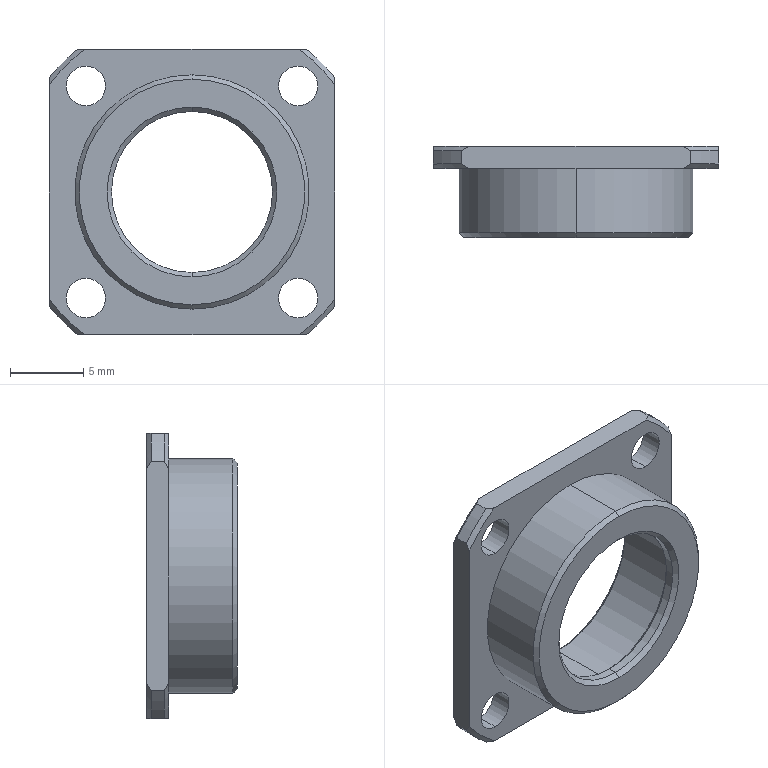Part | SolidWorks | features ICE 2, Revolution 1 | 1 solid | 42 faces | box 19.5 x 6.2 x 19.5 mm | volume 684.644 mm3 | cylinder 18 | cone 16 | plane 8 | commonest cylinder face diameters 2.7 x8 25 x4 11 x2 13 x2 16 x2
STEP:
#1=CARTESIAN_POINT('',(-7.25,4.7,8.6));
#2=VERTEX_POINT('',#1);
#3=CARTESIAN_POINT('',(-7.25,4.7,5.9));
#4=VERTEX_POINT('',#3);
#5=CARTESIAN_POINT('',(-7.25,4.7,7.25));
#6=DIRECTION('',(0.,-1.,0.));
#7=DIRECTION('',(0.,0.,-1.));
#8=AXIS2_PLACEMENT_3D('',#5,#6,#7);
#9=CIRCLE('',#8,1.35);
#10=EDGE_CURVE('',#2,#4,#9,.T.);
#11=ORIENTED_EDGE('',*,*,#10,.T.);
#12=CARTESIAN_POINT('',(-7.25,6.2,5.9));
#13=VERTEX_POINT('',#12);
#14=CARTESIAN_POINT('',(-7.25,-3.8,5.9));
#15=DIRECTION('',(0.,1.,0.));
#16=VECTOR('',#15,1000.);
#17=LINE('',#14,#16);
#18=EDGE_CURVE('',#4,#13,#17,.T.);
#19=ORIENTED_EDGE('',*,*,#18,.T.);
#20=CARTESIAN_POINT('',(-7.25,6.2,8.6));
#21=VERTEX_POINT('',#20);
#22=CARTESIAN_POINT('',(-7.25,6.2,7.25));
#23=DIRECTION('',(0.,1.,0.));
#24=DIRECTION('',(0.,0.,-1.));
#25=AXIS2_PLACEMENT_3D('',#22,#23,#24);
#26=CIRCLE('',#25,1.35);
#27=EDGE_CURVE('',#13,#21,#26,.T.);
#28=ORIENTED_EDGE('',*,*,#27,.T.);
#29=CARTESIAN_POINT('',(-7.25,-3.8,8.6));
#30=DIRECTION('',(0.,1.,0.));
#31=VECTOR('',#30,1000.);
#32=LINE('',#29,#31);
#33=EDGE_CURVE('',#2,#21,#32,.T.);
#34=ORIENTED_EDGE('',*,*,#33,.F.);
#35=EDGE_LOOP('',(#11,#19,#28,#34));
#36=FACE_OUTER_BOUND('',#35,.T.);
#37=CARTESIAN_POINT('',(-7.25,-3.8,7.25));
#38=DIRECTION('',(0.,1.,0.));
#39=DIRECTION('',(0.,0.,1.));
#40=AXIS2_PLACEMENT_3D('',#37,#38,#39);
#41=CYLINDRICAL_SURFACE('',#40,1.35);
#42=ADVANCED_FACE('',(#36),#41,.F.);
#43=CARTESIAN_POINT('',(7.25,4.7,8.6));
#44=VERTEX_POINT('',#43);
#45=CARTESIAN_POINT('',(7.25,4.7,5.9));
#46=VERTEX_POINT('',#45);
#47=CARTESIAN_POINT('',(7.25,4.7,7.25));
#48=DIRECTION('',(0.,-1.,0.));
#49=DIRECTION('',(0.,0.,-1.));
#50=AXIS2_PLACEMENT_3D('',#47,#48,#49);
#51=CIRCLE('',#50,1.35);
#52=EDGE_CURVE('',#44,#46,#51,.T.);
#53=ORIENTED_EDGE('',*,*,#52,.T.);
#54=CARTESIAN_POINT('',(7.25,6.2,5.9));
#55=VERTEX_POINT('',#54);
#56=CARTESIAN_POINT('',(7.25,-3.8,5.9));
#57=DIRECTION('',(0.,1.,0.));
#58=VECTOR('',#57,1000.);
#59=LINE('',#56,#58);
#60=EDGE_CURVE('',#46,#55,#59,.T.);
#61=ORIENTED_EDGE('',*,*,#60,.T.);
#62=CARTESIAN_POINT('',(7.25,6.2,8.6));
#63=VERTEX_POINT('',#62);
#64=CARTESIAN_POINT('',(7.25,6.2,7.25));
#65=DIRECTION('',(0.,1.,0.));
#66=DIRECTION('',(0.,0.,1.));
#67=AXIS2_PLACEMENT_3D('',#64,#65,#66);
#68=CIRCLE('',#67,1.35);
#69=EDGE_CURVE('',#55,#63,#68,.T.);
#70=ORIENTED_EDGE('',*,*,#69,.T.);
#71=CARTESIAN_POINT('',(7.25,-3.8,8.6));
#72=DIRECTION('',(0.,1.,0.));
#73=VECTOR('',#72,1000.);
#74=LINE('',#71,#73);
#75=EDGE_CURVE('',#44,#63,#74,.T.);
#76=ORIENTED_EDGE('',*,*,#75,.F.);
#77=EDGE_LOOP('',(#53,#61,#70,#76));
#78=FACE_OUTER_BOUND('',#77,.T.);
#79=CARTESIAN_POINT('',(7.25,-3.8,7.25));
#80=DIRECTION('',(0.,1.,0.));
#81=DIRECTION('',(0.,0.,1.));
#82=AXIS2_PLACEMENT_3D('',#79,#80,#81);
#83=CYLINDRICAL_SURFACE('',#82,1.35);
#84=ADVANCED_FACE('',(#78),#83,.F.);
#85=CARTESIAN_POINT('',(7.25,4.7,-5.9));
#86=VERTEX_POINT('',#85);
#87=CARTESIAN_POINT('',(7.25,4.7,-8.6));
#88=VERTEX_POINT('',#87);
#89=CARTESIAN_POINT('',(7.25,4.7,-7.25));
#90=DIRECTION('',(0.,-1.,0.));
#91=DIRECTION('',(0.,0.,-1.));
#92=AXIS2_PLACEMENT_3D('',#89,#90,#91);
#93=CIRCLE('',#92,1.35);
#94=EDGE_CURVE('',#86,#88,#93,.T.);
#95=ORIENTED_EDGE('',*,*,#94,.T.);
#96=CARTESIAN_POINT('',(7.25,6.2,-8.6));
#97=VERTEX_POINT('',#96);
#98=CARTESIAN_POINT('',(7.25,-3.8,-8.6));
#99=DIRECTION('',(0.,1.,0.));
#100=VECTOR('',#99,1000.);
#101=LINE('',#98,#100);
#102=EDGE_CURVE('',#88,#97,#101,.T.);
#103=ORIENTED_EDGE('',*,*,#102,.T.);
#104=CARTESIAN_POINT('',(7.25,6.2,-5.9));
#105=VERTEX_POINT('',#104);
#106=CARTESIAN_POINT('',(7.25,6.2,-7.25));
#107=DIRECTION('',(0.,1.,0.));
#108=DIRECTION('',(0.,0.,-1.));
#109=AXIS2_PLACEMENT_3D('',#106,#107,#108);
#110=CIRCLE('',#109,1.35);
#111=EDGE_CURVE('',#97,#105,#110,.T.);
#112=ORIENTED_EDGE('',*,*,#111,.T.);
#113=CARTESIAN_POINT('',(7.25,-3.8,-5.9));
#114=DIRECTION('',(0.,1.,0.));
#115=VECTOR('',#114,1000.);
#116=LINE('',#113,#115);
#117=EDGE_CURVE('',#86,#105,#116,.T.);
#118=ORIENTED_EDGE('',*,*,#117,.F.);
#119=EDGE_LOOP('',(#95,#103,#112,#118));
#120=FACE_OUTER_BOUND('',#119,.T.);
#121=CARTESIAN_POINT('',(7.25,-3.8,-7.25));
#122=DIRECTION('',(0.,1.,0.));
#123=DIRECTION('',(0.,0.,1.));
#124=AXIS2_PLACEMENT_3D('',#121,#122,#123);
#125=CYLINDRICAL_SURFACE('',#124,1.35);
#126=ADVANCED_FACE('',(#120),#125,.F.);
#127=CARTESIAN_POINT('',(-7.25,4.7,-5.9));
#128=VERTEX_POINT('',#127);
#129=CARTESIAN_POINT('',(-7.25,4.7,-8.6));
#130=VERTEX_POINT('',#129);
#131=CARTESIAN_POINT('',(-7.25,4.7,-7.25));
#132=DIRECTION('',(0.,-1.,0.));
#133=DIRECTION('',(0.,0.,-1.));
#134=AXIS2_PLACEMENT_3D('',#131,#132,#133);
#135=CIRCLE('',#134,1.35);
#136=EDGE_CURVE('',#128,#130,#135,.T.);
#137=ORIENTED_EDGE('',*,*,#136,.T.);
#138=CARTESIAN_POINT('',(-7.25,6.2,-8.6));
#139=VERTEX_POINT('',#138);
#140=CARTESIAN_POINT('',(-7.25,-3.8,-8.6));
#141=DIRECTION('',(0.,1.,0.));
#142=VECTOR('',#141,1000.);
#143=LINE('',#140,#142);
#144=EDGE_CURVE('',#130,#139,#143,.T.);
#145=ORIENTED_EDGE('',*,*,#144,.T.);
#146=CARTESIAN_POINT('',(-7.25,6.2,-5.9));
#147=VERTEX_POINT('',#146);
#148=CARTESIAN_POINT('',(-7.25,6.2,-7.25));
#149=DIRECTION('',(0.,1.,0.));
#150=DIRECTION('',(0.,0.,1.));
#151=AXIS2_PLACEMENT_3D('',#148,#149,#150);
#152=CIRCLE('',#151,1.35);
#153=EDGE_CURVE('',#139,#147,#152,.T.);
#154=ORIENTED_EDGE('',*,*,#153,.T.);
#155=CARTESIAN_POINT('',(-7.25,-3.8,-5.9));
#156=DIRECTION('',(0.,1.,0.));
#157=VECTOR('',#156,1000.);
#158=LINE('',#155,#157);
#159=EDGE_CURVE('',#128,#147,#158,.T.);
#160=ORIENTED_EDGE('',*,*,#159,.F.);
#161=EDGE_LOOP('',(#137,#145,#154,#160));
#162=FACE_OUTER_BOUND('',#161,.T.);
#163=CARTESIAN_POINT('',(-7.25,-3.8,-7.25));
#164=DIRECTION('',(0.,1.,0.));
#165=DIRECTION('',(0.,0.,1.));
#166=AXIS2_PLACEMENT_3D('',#163,#164,#165);
#167=CYLINDRICAL_SURFACE('',#166,1.35);
#168=ADVANCED_FACE('',(#162),#167,.F.);
#169=CARTESIAN_POINT('',(0.,4.7,-8.));
#170=VERTEX_POINT('',#169);
#171=CARTESIAN_POINT('',(0.,4.7,8.));
#172=VERTEX_POINT('',#171);
#173=CARTESIAN_POINT('',(0.,4.7,0.));
#174=DIRECTION('',(0.,-1.,0.));
#175=DIRECTION('',(0.,0.,-1.));
#176=AXIS2_PLACEMENT_3D('',#173,#174,#175);
#177=CIRCLE('',#176,8.);
#178=EDGE_CURVE('',#170,#172,#177,.T.);
#179=ORIENTED_EDGE('',*,*,#178,.T.);
#180=CARTESIAN_POINT('',(0.,0.3,8.));
#181=VERTEX_POINT('',#180);
#182=CARTESIAN_POINT('',(0.,0.,8.));
#183=DIRECTION('',(0.,-1.,0.));
#184=VECTOR('',#183,1000.);
#185=LINE('',#182,#184);
#186=EDGE_CURVE('',#172,#181,#185,.T.);
#187=ORIENTED_EDGE('',*,*,#186,.T.);
#188=CARTESIAN_POINT('',(0.,0.3,-8.));
#189=VERTEX_POINT('',#188);
#190=CARTESIAN_POINT('',(0.,0.3,0.));
#191=DIRECTION('',(0.,-1.,0.));
#192=DIRECTION('',(0.,0.,-1.));
#193=AXIS2_PLACEMENT_3D('',#190,#191,#192);
#194=CIRCLE('',#193,8.);
#195=EDGE_CURVE('',#189,#181,#194,.T.);
#196=ORIENTED_EDGE('',*,*,#195,.F.);
#197=CARTESIAN_POINT('',(0.,0.,-8.));
#198=DIRECTION('',(0.,-1.,0.));
#199=VECTOR('',#198,1000.);
#200=LINE('',#197,#199);
#201=EDGE_CURVE('',#170,#189,#200,.T.);
#202=ORIENTED_EDGE('',*,*,#201,.F.);
#203=EDGE_LOOP('',(#179,#187,#196,#202));
#204=FACE_OUTER_BOUND('',#203,.T.);
#205=CARTESIAN_POINT('',(0.,0.,0.));
#206=DIRECTION('',(0.,-1.,0.));
#207=DIRECTION('',(0.,0.,-1.));
#208=AXIS2_PLACEMENT_3D('',#205,#206,#207);
#209=CYLINDRICAL_SURFACE('',#208,8.);
#210=ADVANCED_FACE('',(#204),#209,.T.);
#211=CARTESIAN_POINT('',(0.,0.,-7.7));
#212=VERTEX_POINT('',#211);
#213=CARTESIAN_POINT('',(0.,0.,7.7));
#214=VERTEX_POINT('',#213);
#215=CARTESIAN_POINT('',(0.,0.,0.));
#216=DIRECTION('',(0.,-1.,0.));
#217=DIRECTION('',(0.,0.,-1.));
#218=AXIS2_PLACEMENT_3D('',#215,#216,#217);
#219=CIRCLE('',#218,7.7);
#220=EDGE_CURVE('',#212,#214,#219,.T.);
#221=ORIENTED_EDGE('',*,*,#220,.F.);
#222=CARTESIAN_POINT('',(0.,0.,-7.7));
#223=DIRECTION('',(0.,0.7071,-0.7071));
#224=VECTOR('',#223,1000.);
#225=LINE('',#222,#224);
#226=EDGE_CURVE('',#212,#189,#225,.T.);
#227=ORIENTED_EDGE('',*,*,#226,.T.);
#228=ORIENTED_EDGE('',*,*,#195,.T.);
#229=CARTESIAN_POINT('',(0.,0.,7.7));
#230=DIRECTION('',(0.,0.7071,0.7071));
#231=VECTOR('',#230,1000.);
#232=LINE('',#229,#231);
#233=EDGE_CURVE('',#214,#181,#232,.T.);
#234=ORIENTED_EDGE('',*,*,#233,.F.);
#235=EDGE_LOOP('',(#221,#227,#228,#234));
#236=FACE_OUTER_BOUND('',#235,.T.);
#237=CARTESIAN_POINT('',(0.,0.,0.));
#238=DIRECTION('',(0.,1.,0.));
#239=DIRECTION('',(0.,0.,1.));
#240=AXIS2_PLACEMENT_3D('',#237,#238,#239);
#241=CONICAL_SURFACE('',#240,7.7,0.7854);
#242=ADVANCED_FACE('',(#236),#241,.T.);
#243=CARTESIAN_POINT('',(0.,0.3,5.5));
#244=VERTEX_POINT('',#243);
#245=CARTESIAN_POINT('',(0.,0.3,-5.5));
#246=VERTEX_POINT('',#245);
#247=CARTESIAN_POINT('',(0.,0.3,0.));
#248=DIRECTION('',(0.,-1.,0.));
#249=DIRECTION('',(0.,0.,-1.));
#250=AXIS2_PLACEMENT_3D('',#247,#248,#249);
#251=CIRCLE('',#250,5.5);
#252=EDGE_CURVE('',#244,#246,#251,.T.);
#253=ORIENTED_EDGE('',*,*,#252,.F.);
#254=CARTESIAN_POINT('',(0.,0.,5.8));
#255=VERTEX_POINT('',#254);
#256=CARTESIAN_POINT('',(0.,0.3,5.5));
#257=DIRECTION('',(0.,-0.7071,0.7071));
#258=VECTOR('',#257,1000.);
#259=LINE('',#256,#258);
#260=EDGE_CURVE('',#244,#255,#259,.T.);
#261=ORIENTED_EDGE('',*,*,#260,.T.);
#262=CARTESIAN_POINT('',(0.,0.,-5.8));
#263=VERTEX_POINT('',#262);
#264=CARTESIAN_POINT('',(0.,0.,0.));
#265=DIRECTION('',(0.,-1.,0.));
#266=DIRECTION('',(0.,0.,-1.));
#267=AXIS2_PLACEMENT_3D('',#264,#265,#266);
#268=CIRCLE('',#267,5.8);
#269=EDGE_CURVE('',#255,#263,#268,.T.);
#270=ORIENTED_EDGE('',*,*,#269,.T.);
#271=CARTESIAN_POINT('',(0.,0.3,-5.5));
#272=DIRECTION('',(0.,-0.7071,-0.7071));
#273=VECTOR('',#272,1000.);
#274=LINE('',#271,#273);
#275=EDGE_CURVE('',#246,#263,#274,.T.);
#276=ORIENTED_EDGE('',*,*,#275,.F.);
#277=EDGE_LOOP('',(#253,#261,#270,#276));
#278=FACE_OUTER_BOUND('',#277,.T.);
#279=CARTESIAN_POINT('',(0.,0.3,0.));
#280=DIRECTION('',(0.,-1.,0.));
#281=DIRECTION('',(0.,0.,-1.));
#282=AXIS2_PLACEMENT_3D('',#279,#280,#281);
#283=CONICAL_SURFACE('',#282,5.5,0.7854);
#284=ADVANCED_FACE('',(#278),#283,.F.);
#285=CARTESIAN_POINT('',(0.,0.9,5.5));
#286=VERTEX_POINT('',#285);
#287=CARTESIAN_POINT('',(0.,0.9,-5.5));
#288=VERTEX_POINT('',#287);
#289=CARTESIAN_POINT('',(0.,0.9,0.));
#290=DIRECTION('',(0.,-1.,0.));
#291=DIRECTION('',(0.,0.,-1.));
#292=AXIS2_PLACEMENT_3D('',#289,#290,#291);
#293=CIRCLE('',#292,5.5);
#294=EDGE_CURVE('',#286,#288,#293,.T.);
#295=ORIENTED_EDGE('',*,*,#294,.F.);
#296=CARTESIAN_POINT('',(0.,0.,5.5));
#297=DIRECTION('',(0.,-1.,0.));
#298=VECTOR('',#297,1000.);
#299=LINE('',#296,#298);
#300=EDGE_CURVE('',#286,#244,#299,.T.);
#301=ORIENTED_EDGE('',*,*,#300,.T.);
#302=ORIENTED_EDGE('',*,*,#252,.T.);
#303=CARTESIAN_POINT('',(0.,0.,-5.5));
#304=DIRECTION('',(0.,-1.,0.));
#305=VECTOR('',#304,1000.);
#306=LINE('',#303,#305);
#307=EDGE_CURVE('',#288,#246,#306,.T.);
#308=ORIENTED_EDGE('',*,*,#307,.F.);
#309=EDGE_LOOP('',(#295,#301,#302,#308));
#310=FACE_OUTER_BOUND('',#309,.T.);
#311=CARTESIAN_POINT('',(0.,0.,0.));
#312=DIRECTION('',(0.,-1.,0.));
#313=DIRECTION('',(0.,0.,-1.));
#314=AXIS2_PLACEMENT_3D('',#311,#312,#313);
#315=CYLINDRICAL_SURFACE('',#314,5.5);
#316=ADVANCED_FACE('',(#310),#315,.F.);
#317=ORIENTED_EDGE('',*,*,#294,.T.);
#318=CARTESIAN_POINT('',(0.,1.2,-5.8));
#319=VERTEX_POINT('',#318);
#320=CARTESIAN_POINT('',(0.,1.2,-5.8));
#321=DIRECTION('',(0.,0.7071,-0.7071));
#322=VECTOR('',#321,1000.);
#323=LINE('',#320,#322);
#324=EDGE_CURVE('',#288,#319,#323,.T.);
#325=ORIENTED_EDGE('',*,*,#324,.T.);
#326=CARTESIAN_POINT('',(0.,1.2,5.8));
#327=VERTEX_POINT('',#326);
#328=CARTESIAN_POINT('',(0.,1.2,0.));
#329=DIRECTION('',(0.,-1.,0.));
#330=DIRECTION('',(0.,0.,-1.));
#331=AXIS2_PLACEMENT_3D('',#328,#329,#330);
#332=CIRCLE('',#331,5.8);
#333=EDGE_CURVE('',#327,#319,#332,.T.);
#334=ORIENTED_EDGE('',*,*,#333,.F.);
#335=CARTESIAN_POINT('',(0.,1.2,5.8));
#336=DIRECTION('',(0.,0.7071,0.7071));
#337=VECTOR('',#336,1000.);
#338=LINE('',#335,#337);
#339=EDGE_CURVE('',#286,#327,#338,.T.);
#340=ORIENTED_EDGE('',*,*,#339,.F.);
#341=EDGE_LOOP('',(#317,#325,#334,#340));
#342=FACE_OUTER_BOUND('',#341,.T.);
#343=CARTESIAN_POINT('',(0.,1.2,0.));
#344=DIRECTION('',(0.,1.,0.));
#345=DIRECTION('',(0.,0.,1.));
#346=AXIS2_PLACEMENT_3D('',#343,#344,#345);
#347=CONICAL_SURFACE('',#346,5.8,0.7854);
#348=ADVANCED_FACE('',(#342),#347,.F.);
#349=CARTESIAN_POINT('',(0.,5.9,6.5));
#350=VERTEX_POINT('',#349);
#351=CARTESIAN_POINT('',(0.,5.9,-6.5));
#352=VERTEX_POINT('',#351);
#353=CARTESIAN_POINT('',(0.,5.9,0.));
#354=DIRECTION('',(0.,-1.,0.));
#355=DIRECTION('',(0.,0.,-1.));
#356=AXIS2_PLACEMENT_3D('',#353,#354,#355);
#357=CIRCLE('',#356,6.5);
#358=EDGE_CURVE('',#350,#352,#357,.T.);
#359=ORIENTED_EDGE('',*,*,#358,.F.);
#360=CARTESIAN_POINT('',(0.,1.2,6.5));
#361=VERTEX_POINT('',#360);
#362=CARTESIAN_POINT('',(0.,0.,6.5));
#363=DIRECTION('',(0.,-1.,0.));
#364=VECTOR('',#363,1000.);
#365=LINE('',#362,#364);
#366=EDGE_CURVE('',#350,#361,#365,.T.);
#367=ORIENTED_EDGE('',*,*,#366,.T.);
#368=CARTESIAN_POINT('',(0.,1.2,-6.5));
#369=VERTEX_POINT('',#368);
#370=CARTESIAN_POINT('',(0.,1.2,0.));
#371=DIRECTION('',(0.,-1.,0.));
#372=DIRECTION('',(0.,0.,-1.));
#373=AXIS2_PLACEMENT_3D('',#370,#371,#372);
#374=CIRCLE('',#373,6.5);
#375=EDGE_CURVE('',#361,#369,#374,.T.);
#376=ORIENTED_EDGE('',*,*,#375,.T.);
#377=CARTESIAN_POINT('',(0.,0.,-6.5));
#378=DIRECTION('',(0.,-1.,0.));
#379=VECTOR('',#378,1000.);
#380=LINE('',#377,#379);
#381=EDGE_CURVE('',#352,#369,#380,.T.);
#382=ORIENTED_EDGE('',*,*,#381,.F.);
#383=EDGE_LOOP('',(#359,#367,#376,#382));
#384=FACE_OUTER_BOUND('',#383,.T.);
#385=CARTESIAN_POINT('',(0.,0.,0.));
#386=DIRECTION('',(0.,-1.,0.));
#387=DIRECTION('',(0.,0.,-1.));
#388=AXIS2_PLACEMENT_3D('',#385,#386,#387);
#389=CYLINDRICAL_SURFACE('',#388,6.5);
#390=ADVANCED_FACE('',(#384),#389,.F.);
#391=ORIENTED_EDGE('',*,*,#358,.T.);
#392=CARTESIAN_POINT('',(0.,6.2,-6.8));
#393=VERTEX_POINT('',#392);
#394=CARTESIAN_POINT('',(0.,6.2,-6.8));
#395=DIRECTION('',(0.,0.7071,-0.7071));
#396=VECTOR('',#395,1000.);
#397=LINE('',#394,#396);
#398=EDGE_CURVE('',#352,#393,#397,.T.);
#399=ORIENTED_EDGE('',*,*,#398,.T.);
#400=CARTESIAN_POINT('',(0.,6.2,6.8));
#401=VERTEX_POINT('',#400);
#402=CARTESIAN_POINT('',(0.,6.2,0.));
#403=DIRECTION('',(0.,-1.,0.));
#404=DIRECTION('',(0.,0.,-1.));
#405=AXIS2_PLACEMENT_3D('',#402,#403,#404);
#406=CIRCLE('',#405,6.8);
#407=EDGE_CURVE('',#401,#393,#406,.T.);
#408=ORIENTED_EDGE('',*,*,#407,.F.);
#409=CARTESIAN_POINT('',(0.,6.2,6.8));
#410=DIRECTION('',(0.,0.7071,0.7071));
#411=VECTOR('',#410,1000.);
#412=LINE('',#409,#411);
#413=EDGE_CURVE('',#350,#401,#412,.T.);
#414=ORIENTED_EDGE('',*,*,#413,.F.);
#415=EDGE_LOOP('',(#391,#399,#408,#414));
#416=FACE_OUTER_BOUND('',#415,.T.);
#417=CARTESIAN_POINT('',(0.,6.2,0.));
#418=DIRECTION('',(0.,1.,0.));
#419=DIRECTION('',(0.,0.,1.));
#420=AXIS2_PLACEMENT_3D('',#417,#418,#419);
#421=CONICAL_SURFACE('',#420,6.8,0.7854);
#422=ADVANCED_FACE('',(#416),#421,.F.);
#423=ORIENTED_EDGE('',*,*,#10,.F.);
#424=CARTESIAN_POINT('',(-7.25,4.7,7.25));
#425=DIRECTION('',(0.,-1.,0.));
#426=DIRECTION('',(0.,0.,-1.));
#427=AXIS2_PLACEMENT_3D('',#424,#425,#426);
#428=CIRCLE('',#427,1.35);
#429=EDGE_CURVE('',#4,#2,#428,.T.);
#430=ORIENTED_EDGE('',*,*,#429,.F.);
#431=EDGE_LOOP('',(#423,#430));
#432=FACE_BOUND('',#431,.T.);
#433=ORIENTED_EDGE('',*,*,#52,.F.);
#434=CARTESIAN_POINT('',(7.25,4.7,7.25));
#435=DIRECTION('',(0.,-1.,0.));
#436=DIRECTION('',(0.,0.,-1.));
#437=AXIS2_PLACEMENT_3D('',#434,#435,#436);
#438=CIRCLE('',#437,1.35);
#439=EDGE_CURVE('',#46,#44,#438,.T.);
#440=ORIENTED_EDGE('',*,*,#439,.F.);
#441=EDGE_LOOP('',(#433,#440));
#442=FACE_BOUND('',#441,.T.);
#443=ORIENTED_EDGE('',*,*,#94,.F.);
#444=CARTESIAN_POINT('',(7.25,4.7,-7.25));
#445=DIRECTION('',(0.,-1.,0.));
#446=DIRECTION('',(0.,0.,-1.));
#447=AXIS2_PLACEMENT_3D('',#444,#445,#446);
#448=CIRCLE('',#447,1.35);
#449=EDGE_CURVE('',#88,#86,#448,.T.);
#450=ORIENTED_EDGE('',*,*,#449,.F.);
#451=EDGE_LOOP('',(#443,#450));
#452=FACE_BOUND('',#451,.T.);
#453=ORIENTED_EDGE('',*,*,#136,.F.);
#454=CARTESIAN_POINT('',(-7.25,4.7,-7.25));
#455=DIRECTION('',(0.,-1.,0.));
#456=DIRECTION('',(0.,0.,-1.));
#457=AXIS2_PLACEMENT_3D('',#454,#455,#456);
#458=CIRCLE('',#457,1.35);
#459=EDGE_CURVE('',#130,#128,#458,.T.);
#460=ORIENTED_EDGE('',*,*,#459,.F.);
#461=EDGE_LOOP('',(#453,#460));
#462=FACE_BOUND('',#461,.T.);
#463=ORIENTED_EDGE('',*,*,#178,.F.);
#464=CARTESIAN_POINT('',(0.,4.7,0.));
#465=DIRECTION('',(0.,-1.,0.));
#466=DIRECTION('',(0.,0.,-1.));
#467=AXIS2_PLACEMENT_3D('',#464,#465,#466);
#468=CIRCLE('',#467,8.);
#469=EDGE_CURVE('',#172,#170,#468,.T.);
#470=ORIENTED_EDGE('',*,*,#469,.F.);
#471=EDGE_LOOP('',(#463,#470));
#472=FACE_BOUND('',#471,.T.);
#473=CARTESIAN_POINT('',(7.333,4.7,-9.75));
#474=VERTEX_POINT('',#473);
#475=CARTESIAN_POINT('',(9.75,4.7,-7.333));
#476=VERTEX_POINT('',#475);
#477=CARTESIAN_POINT('',(0.,4.7,0.));
#478=DIRECTION('',(0.,-1.,0.));
#479=DIRECTION('',(0.,0.,-1.));
#480=AXIS2_PLACEMENT_3D('',#477,#478,#479);
#481=CIRCLE('',#480,12.2);
#482=EDGE_CURVE('',#474,#476,#481,.T.);
#483=ORIENTED_EDGE('',*,*,#482,.T.);
#484=CARTESIAN_POINT('',(9.75,4.7,7.333));
#485=VERTEX_POINT('',#484);
#486=CARTESIAN_POINT('',(9.75,4.7,0.));
#487=DIRECTION('',(0.,0.,1.));
#488=VECTOR('',#487,1000.);
#489=LINE('',#486,#488);
#490=EDGE_CURVE('',#476,#485,#489,.T.);
#491=ORIENTED_EDGE('',*,*,#490,.T.);
#492=CARTESIAN_POINT('',(7.333,4.7,9.75));
#493=VERTEX_POINT('',#492);
#494=CARTESIAN_POINT('',(0.,4.7,0.));
#495=DIRECTION('',(0.,-1.,0.));
#496=DIRECTION('',(0.,0.,-1.));
#497=AXIS2_PLACEMENT_3D('',#494,#495,#496);
#498=CIRCLE('',#497,12.2);
#499=EDGE_CURVE('',#485,#493,#498,.T.);
#500=ORIENTED_EDGE('',*,*,#499,.T.);
#501=CARTESIAN_POINT('',(-7.333,4.7,9.75));
#502=VERTEX_POINT('',#501);
#503=CARTESIAN_POINT('',(8.,4.7,9.75));
#504=DIRECTION('',(-1.,0.,0.));
#505=VECTOR('',#504,1000.);
#506=LINE('',#503,#505);
#507=EDGE_CURVE('',#493,#502,#506,.T.);
#508=ORIENTED_EDGE('',*,*,#507,.T.);
#509=CARTESIAN_POINT('',(-9.75,4.7,7.333));
#510=VERTEX_POINT('',#509);
#511=CARTESIAN_POINT('',(0.,4.7,0.));
#512=DIRECTION('',(0.,-1.,0.));
#513=DIRECTION('',(0.,0.,-1.));
#514=AXIS2_PLACEMENT_3D('',#511,#512,#513);
#515=CIRCLE('',#514,12.2);
#516=EDGE_CURVE('',#502,#510,#515,.T.);
#517=ORIENTED_EDGE('',*,*,#516,.T.);
#518=CARTESIAN_POINT('',(-9.75,4.7,-7.333));
#519=VERTEX_POINT('',#518);
#520=CARTESIAN_POINT('',(-9.75,4.7,0.));
#521=DIRECTION('',(0.,0.,-1.));
#522=VECTOR('',#521,1000.);
#523=LINE('',#520,#522);
#524=EDGE_CURVE('',#510,#519,#523,.T.);
#525=ORIENTED_EDGE('',*,*,#524,.T.);
#526=CARTESIAN_POINT('',(-7.333,4.7,-9.75));
#527=VERTEX_POINT('',#526);
#528=CARTESIAN_POINT('',(0.,4.7,0.));
#529=DIRECTION('',(0.,-1.,0.));
#530=DIRECTION('',(0.,0.,-1.));
#531=AXIS2_PLACEMENT_3D('',#528,#529,#530);
#532=CIRCLE('',#531,12.2);
#533=EDGE_CURVE('',#519,#527,#532,.T.);
#534=ORIENTED_EDGE('',*,*,#533,.T.);
#535=CARTESIAN_POINT('',(8.,4.7,-9.75));
#536=DIRECTION('',(1.,0.,0.));
#537=VECTOR('',#536,1000.);
#538=LINE('',#535,#537);
#539=EDGE_CURVE('',#527,#474,#538,.T.);
#540=ORIENTED_EDGE('',*,*,#539,.T.);
#541=EDGE_LOOP('',(#483,#491,#500,#508,#517,#525,#534,#540));
#542=FACE_OUTER_BOUND('',#541,.T.);
#543=CARTESIAN_POINT('',(8.,4.7,0.));
#544=DIRECTION('',(0.,-1.,0.));
#545=DIRECTION('',(0.,0.,-1.));
#546=AXIS2_PLACEMENT_3D('',#543,#544,#545);
#547=PLANE('',#546);
#548=ADVANCED_FACE('',(#432,#442,#452,#462,#472,#542),#547,.T.);
#549=CARTESIAN_POINT('',(7.822,5.,-9.75));
#550=VERTEX_POINT('',#549);
#551=CARTESIAN_POINT('',(9.75,5.,-7.822));
#552=VERTEX_POINT('',#551);
#553=CARTESIAN_POINT('',(0.,5.,0.));
#554=DIRECTION('',(0.,-1.,0.));
#555=DIRECTION('',(0.,0.,-1.));
#556=AXIS2_PLACEMENT_3D('',#553,#554,#555);
#557=CIRCLE('',#556,12.5);
#558=EDGE_CURVE('',#550,#552,#557,.T.);
#559=ORIENTED_EDGE('',*,*,#558,.T.);
#560=CARTESIAN_POINT('',(9.75,5.,-7.822));
#561=CARTESIAN_POINT('',(9.75,4.899,-7.66));
#562=CARTESIAN_POINT('',(9.75,4.799,-7.497));
#563=CARTESIAN_POINT('',(9.75,4.7,-7.333));
#564=B_SPLINE_CURVE_WITH_KNOTS('',3,(#560,#561,#562,#563),.UNSPECIFIED.,.F.,.F.,(4,4),(0.01758,0.01815),.UNSPECIFIED.);
#565=EDGE_CURVE('',#552,#476,#564,.T.);
#566=ORIENTED_EDGE('',*,*,#565,.T.);
#567=ORIENTED_EDGE('',*,*,#482,.F.);
#568=CARTESIAN_POINT('',(7.333,4.7,-9.75));
#569=CARTESIAN_POINT('',(7.497,4.799,-9.75));
#570=CARTESIAN_POINT('',(7.66,4.899,-9.75));
#571=CARTESIAN_POINT('',(7.822,5.,-9.75));
#572=B_SPLINE_CURVE_WITH_KNOTS('',3,(#568,#569,#570,#571),.UNSPECIFIED.,.F.,.F.,(4,4),(0.03382,0.0344),.UNSPECIFIED.);
#573=EDGE_CURVE('',#474,#550,#572,.T.);
#574=ORIENTED_EDGE('',*,*,#573,.T.);
#575=EDGE_LOOP('',(#559,#566,#567,#574));
#576=FACE_OUTER_BOUND('',#575,.T.);
#577=CARTESIAN_POINT('',(0.,4.7,0.));
#578=DIRECTION('',(0.,1.,0.));
#579=DIRECTION('',(0.,0.,1.));
#580=AXIS2_PLACEMENT_3D('',#577,#578,#579);
#581=CONICAL_SURFACE('',#580,12.2,0.7854);
#582=ADVANCED_FACE('',(#576),#581,.T.);
#583=ORIENTED_EDGE('',*,*,#499,.F.);
#584=CARTESIAN_POINT('',(9.75,5.,7.822));
#585=VERTEX_POINT('',#584);
#586=CARTESIAN_POINT('',(9.75,4.7,7.333));
#587=CARTESIAN_POINT('',(9.75,4.799,7.497));
#588=CARTESIAN_POINT('',(9.75,4.899,7.66));
#589=CARTESIAN_POINT('',(9.75,5.,7.822));
#590=B_SPLINE_CURVE_WITH_KNOTS('',3,(#586,#587,#588,#589),.UNSPECIFIED.,.F.,.F.,(4,4),(0.03382,0.0344),.UNSPECIFIED.);
#591=EDGE_CURVE('',#485,#585,#590,.T.);
#592=ORIENTED_EDGE('',*,*,#591,.T.);
#593=CARTESIAN_POINT('',(7.822,5.,9.75));
#594=VERTEX_POINT('',#593);
#595=CARTESIAN_POINT('',(0.,5.,0.));
#596=DIRECTION('',(0.,-1.,0.));
#597=DIRECTION('',(0.,0.,-1.));
#598=AXIS2_PLACEMENT_3D('',#595,#596,#597);
#599=CIRCLE('',#598,12.5);
#600=EDGE_CURVE('',#585,#594,#599,.T.);
#601=ORIENTED_EDGE('',*,*,#600,.T.);
#602=CARTESIAN_POINT('',(7.822,5.,9.75));
#603=CARTESIAN_POINT('',(7.66,4.899,9.75));
#604=CARTESIAN_POINT('',(7.497,4.799,9.75));
#605=CARTESIAN_POINT('',(7.333,4.7,9.75));
#606=B_SPLINE_CURVE_WITH_KNOTS('',3,(#602,#603,#604,#605),.UNSPECIFIED.,.F.,.F.,(4,4),(0.01758,0.01815),.UNSPECIFIED.);
#607=EDGE_CURVE('',#594,#493,#606,.T.);
#608=ORIENTED_EDGE('',*,*,#607,.T.);
#609=EDGE_LOOP('',(#583,#592,#601,#608));
#610=FACE_OUTER_BOUND('',#609,.T.);
#611=CARTESIAN_POINT('',(0.,4.7,0.));
#612=DIRECTION('',(0.,1.,0.));
#613=DIRECTION('',(0.,0.,1.));
#614=AXIS2_PLACEMENT_3D('',#611,#612,#613);
#615=CONICAL_SURFACE('',#614,12.2,0.7854);
#616=ADVANCED_FACE('',(#610),#615,.T.);
#617=ORIENTED_EDGE('',*,*,#516,.F.);
#618=CARTESIAN_POINT('',(-7.822,5.,9.75));
#619=VERTEX_POINT('',#618);
#620=CARTESIAN_POINT('',(-7.333,4.7,9.75));
#621=CARTESIAN_POINT('',(-7.497,4.799,9.75));
#622=CARTESIAN_POINT('',(-7.66,4.899,9.75));
#623=CARTESIAN_POINT('',(-7.822,5.,9.75));
#624=B_SPLINE_CURVE_WITH_KNOTS('',3,(#620,#621,#622,#623),.UNSPECIFIED.,.F.,.F.,(4,4),(0.03382,0.0344),.UNSPECIFIED.);
#625=EDGE_CURVE('',#502,#619,#624,.T.);
#626=ORIENTED_EDGE('',*,*,#625,.T.);
#627=CARTESIAN_POINT('',(-9.75,5.,7.822));
#628=VERTEX_POINT('',#627);
#629=CARTESIAN_POINT('',(0.,5.,0.));
#630=DIRECTION('',(0.,-1.,0.));
#631=DIRECTION('',(0.,0.,-1.));
#632=AXIS2_PLACEMENT_3D('',#629,#630,#631);
#633=CIRCLE('',#632,12.5);
#634=EDGE_CURVE('',#619,#628,#633,.T.);
#635=ORIENTED_EDGE('',*,*,#634,.T.);
#636=CARTESIAN_POINT('',(-9.75,5.,7.822));
#637=CARTESIAN_POINT('',(-9.75,4.899,7.66));
#638=CARTESIAN_POINT('',(-9.75,4.799,7.497));
#639=CARTESIAN_POINT('',(-9.75,4.7,7.333));
#640=B_SPLINE_CURVE_WITH_KNOTS('',3,(#636,#637,#638,#639),.UNSPECIFIED.,.F.,.F.,(4,4),(0.01758,0.01815),.UNSPECIFIED.);
#641=EDGE_CURVE('',#628,#510,#640,.T.);
#642=ORIENTED_EDGE('',*,*,#641,.T.);
#643=EDGE_LOOP('',(#617,#626,#635,#642));
#644=FACE_OUTER_BOUND('',#643,.T.);
#645=CARTESIAN_POINT('',(0.,4.7,0.));
#646=DIRECTION('',(0.,1.,0.));
#647=DIRECTION('',(0.,0.,1.));
#648=AXIS2_PLACEMENT_3D('',#645,#646,#647);
#649=CONICAL_SURFACE('',#648,12.2,0.7854);
#650=ADVANCED_FACE('',(#644),#649,.T.);
#651=ORIENTED_EDGE('',*,*,#533,.F.);
#652=CARTESIAN_POINT('',(-9.75,5.,-7.822));
#653=VERTEX_POINT('',#652);
#654=CARTESIAN_POINT('',(-9.75,4.7,-7.333));
#655=CARTESIAN_POINT('',(-9.75,4.799,-7.497));
#656=CARTESIAN_POINT('',(-9.75,4.899,-7.66));
#657=CARTESIAN_POINT('',(-9.75,5.,-7.822));
#658=B_SPLINE_CURVE_WITH_KNOTS('',3,(#654,#655,#656,#657),.UNSPECIFIED.,.F.,.F.,(4,4),(0.03382,0.0344),.UNSPECIFIED.);
#659=EDGE_CURVE('',#519,#653,#658,.T.);
#660=ORIENTED_EDGE('',*,*,#659,.T.);
#661=CARTESIAN_POINT('',(-7.822,5.,-9.75));
#662=VERTEX_POINT('',#661);
#663=CARTESIAN_POINT('',(0.,5.,0.));
#664=DIRECTION('',(0.,-1.,0.));
#665=DIRECTION('',(0.,0.,-1.));
#666=AXIS2_PLACEMENT_3D('',#663,#664,#665);
#667=CIRCLE('',#666,12.5);
#668=EDGE_CURVE('',#653,#662,#667,.T.);
#669=ORIENTED_EDGE('',*,*,#668,.T.);
#670=CARTESIAN_POINT('',(-7.822,5.,-9.75));
#671=CARTESIAN_POINT('',(-7.66,4.899,-9.75));
#672=CARTESIAN_POINT('',(-7.497,4.799,-9.75));
#673=CARTESIAN_POINT('',(-7.333,4.7,-9.75));
#674=B_SPLINE_CURVE_WITH_KNOTS('',3,(#670,#671,#672,#673),.UNSPECIFIED.,.F.,.F.,(4,4),(0.01758,0.01815),.UNSPECIFIED.);
#675=EDGE_CURVE('',#662,#527,#674,.T.);
#676=ORIENTED_EDGE('',*,*,#675,.T.);
#677=EDGE_LOOP('',(#651,#660,#669,#676));
#678=FACE_OUTER_BOUND('',#677,.T.);
#679=CARTESIAN_POINT('',(0.,4.7,0.));
#680=DIRECTION('',(0.,1.,0.));
#681=DIRECTION('',(0.,0.,1.));
#682=AXIS2_PLACEMENT_3D('',#679,#680,#681);
#683=CONICAL_SURFACE('',#682,12.2,0.7854);
#684=ADVANCED_FACE('',(#678),#683,.T.);
#685=ORIENTED_EDGE('',*,*,#600,.F.);
#686=CARTESIAN_POINT('',(9.75,5.9,7.822));
#687=VERTEX_POINT('',#686);
#688=CARTESIAN_POINT('',(9.75,0.,7.822));
#689=DIRECTION('',(0.,1.,0.));
#690=VECTOR('',#689,1000.);
#691=LINE('',#688,#690);
#692=EDGE_CURVE('',#585,#687,#691,.T.);
#693=ORIENTED_EDGE('',*,*,#692,.T.);
#694=CARTESIAN_POINT('',(7.822,5.9,9.75));
#695=VERTEX_POINT('',#694);
#696=CARTESIAN_POINT('',(0.,5.9,0.));
#697=DIRECTION('',(0.,-1.,0.));
#698=DIRECTION('',(0.,0.,-1.));
#699=AXIS2_PLACEMENT_3D('',#696,#697,#698);
#700=CIRCLE('',#699,12.5);
#701=EDGE_CURVE('',#687,#695,#700,.T.);
#702=ORIENTED_EDGE('',*,*,#701,.T.);
#703=CARTESIAN_POINT('',(7.822,0.,9.75));
#704=DIRECTION('',(0.,-1.,0.));
#705=VECTOR('',#704,1000.);
#706=LINE('',#703,#705);
#707=EDGE_CURVE('',#695,#594,#706,.T.);
#708=ORIENTED_EDGE('',*,*,#707,.T.);
#709=EDGE_LOOP('',(#685,#693,#702,#708));
#710=FACE_OUTER_BOUND('',#709,.T.);
#711=CARTESIAN_POINT('',(0.,0.,0.));
#712=DIRECTION('',(0.,-1.,0.));
#713=DIRECTION('',(0.,0.,-1.));
#714=AXIS2_PLACEMENT_3D('',#711,#712,#713);
#715=CYLINDRICAL_SURFACE('',#714,12.5);
#716=ADVANCED_FACE('',(#710),#715,.T.);
#717=CARTESIAN_POINT('',(7.822,5.9,-9.75));
#718=VERTEX_POINT('',#717);
#719=CARTESIAN_POINT('',(9.75,5.9,-7.822));
#720=VERTEX_POINT('',#719);
#721=CARTESIAN_POINT('',(0.,5.9,0.));
#722=DIRECTION('',(0.,-1.,0.));
#723=DIRECTION('',(0.,0.,-1.));
#724=AXIS2_PLACEMENT_3D('',#721,#722,#723);
#725=CIRCLE('',#724,12.5);
#726=EDGE_CURVE('',#718,#720,#725,.T.);
#727=ORIENTED_EDGE('',*,*,#726,.T.);
#728=CARTESIAN_POINT('',(9.75,0.,-7.822));
#729=DIRECTION('',(0.,-1.,0.));
#730=VECTOR('',#729,1000.);
#731=LINE('',#728,#730);
#732=EDGE_CURVE('',#720,#552,#731,.T.);
#733=ORIENTED_EDGE('',*,*,#732,.T.);
#734=ORIENTED_EDGE('',*,*,#558,.F.);
#735=CARTESIAN_POINT('',(7.822,0.,-9.75));
#736=DIRECTION('',(0.,1.,0.));
#737=VECTOR('',#736,1000.);
#738=LINE('',#735,#737);
#739=EDGE_CURVE('',#550,#718,#738,.T.);
#740=ORIENTED_EDGE('',*,*,#739,.T.);
#741=EDGE_LOOP('',(#727,#733,#734,#740));
#742=FACE_OUTER_BOUND('',#741,.T.);
#743=CARTESIAN_POINT('',(0.,0.,0.));
#744=DIRECTION('',(0.,-1.,0.));
#745=DIRECTION('',(0.,0.,-1.));
#746=AXIS2_PLACEMENT_3D('',#743,#744,#745);
#747=CYLINDRICAL_SURFACE('',#746,12.5);
#748=ADVANCED_FACE('',(#742),#747,.T.);
#749=ORIENTED_EDGE('',*,*,#634,.F.);
#750=CARTESIAN_POINT('',(-7.822,5.9,9.75));
#751=VERTEX_POINT('',#750);
#752=CARTESIAN_POINT('',(-7.822,0.,9.75));
#753=DIRECTION('',(0.,1.,0.));
#754=VECTOR('',#753,1000.);
#755=LINE('',#752,#754);
#756=EDGE_CURVE('',#619,#751,#755,.T.);
#757=ORIENTED_EDGE('',*,*,#756,.T.);
#758=CARTESIAN_POINT('',(-9.75,5.9,7.822));
#759=VERTEX_POINT('',#758);
#760=CARTESIAN_POINT('',(0.,5.9,0.));
#761=DIRECTION('',(0.,-1.,0.));
#762=DIRECTION('',(0.,0.,-1.));
#763=AXIS2_PLACEMENT_3D('',#760,#761,#762);
#764=CIRCLE('',#763,12.5);
#765=EDGE_CURVE('',#751,#759,#764,.T.);
#766=ORIENTED_EDGE('',*,*,#765,.T.);
#767=CARTESIAN_POINT('',(-9.75,0.,7.822));
#768=DIRECTION('',(0.,-1.,0.));
#769=VECTOR('',#768,1000.);
#770=LINE('',#767,#769);
#771=EDGE_CURVE('',#759,#628,#770,.T.);
#772=ORIENTED_EDGE('',*,*,#771,.T.);
#773=EDGE_LOOP('',(#749,#757,#766,#772));
#774=FACE_OUTER_BOUND('',#773,.T.);
#775=CARTESIAN_POINT('',(0.,0.,0.));
#776=DIRECTION('',(0.,-1.,0.));
#777=DIRECTION('',(0.,0.,-1.));
#778=AXIS2_PLACEMENT_3D('',#775,#776,#777);
#779=CYLINDRICAL_SURFACE('',#778,12.5);
#780=ADVANCED_FACE('',(#774),#779,.T.);
#781=ORIENTED_EDGE('',*,*,#668,.F.);
#782=CARTESIAN_POINT('',(-9.75,5.9,-7.822));
#783=VERTEX_POINT('',#782);
#784=CARTESIAN_POINT('',(-9.75,0.,-7.822));
#785=DIRECTION('',(0.,1.,0.));
#786=VECTOR('',#785,1000.);
#787=LINE('',#784,#786);
#788=EDGE_CURVE('',#653,#783,#787,.T.);
#789=ORIENTED_EDGE('',*,*,#788,.T.);
#790=CARTESIAN_POINT('',(-7.822,5.9,-9.75));
#791=VERTEX_POINT('',#790);
#792=CARTESIAN_POINT('',(0.,5.9,0.));
#793=DIRECTION('',(0.,-1.,0.));
#794=DIRECTION('',(0.,0.,-1.));
#795=AXIS2_PLACEMENT_3D('',#792,#793,#794);
#796=CIRCLE('',#795,12.5);
#797=EDGE_CURVE('',#783,#791,#796,.T.);
#798=ORIENTED_EDGE('',*,*,#797,.T.);
#799=CARTESIAN_POINT('',(-7.822,0.,-9.75));
#800=DIRECTION('',(0.,-1.,0.));
#801=VECTOR('',#800,1000.);
#802=LINE('',#799,#801);
#803=EDGE_CURVE('',#791,#662,#802,.T.);
#804=ORIENTED_EDGE('',*,*,#803,.T.);
#805=EDGE_LOOP('',(#781,#789,#798,#804));
#806=FACE_OUTER_BOUND('',#805,.T.);
#807=CARTESIAN_POINT('',(0.,0.,0.));
#808=DIRECTION('',(0.,-1.,0.));
#809=DIRECTION('',(0.,0.,-1.));
#810=AXIS2_PLACEMENT_3D('',#807,#808,#809);
#811=CYLINDRICAL_SURFACE('',#810,12.5);
#812=ADVANCED_FACE('',(#806),#811,.T.);
#813=ORIENTED_EDGE('',*,*,#701,.F.);
#814=CARTESIAN_POINT('',(9.75,6.2,7.333));
#815=VERTEX_POINT('',#814);
#816=CARTESIAN_POINT('',(9.75,5.9,7.822));
#817=CARTESIAN_POINT('',(9.75,6.001,7.66));
#818=CARTESIAN_POINT('',(9.75,6.101,7.497));
#819=CARTESIAN_POINT('',(9.75,6.2,7.333));
#820=B_SPLINE_CURVE_WITH_KNOTS('',3,(#816,#817,#818,#819),.UNSPECIFIED.,.F.,.F.,(4,4),(0.01758,0.01815),.UNSPECIFIED.);
#821=EDGE_CURVE('',#687,#815,#820,.T.);
#822=ORIENTED_EDGE('',*,*,#821,.T.);
#823=CARTESIAN_POINT('',(7.333,6.2,9.75));
#824=VERTEX_POINT('',#823);
#825=CARTESIAN_POINT('',(0.,6.2,0.));
#826=DIRECTION('',(0.,-1.,0.));
#827=DIRECTION('',(0.,0.,-1.));
#828=AXIS2_PLACEMENT_3D('',#825,#826,#827);
#829=CIRCLE('',#828,12.2);
#830=EDGE_CURVE('',#815,#824,#829,.T.);
#831=ORIENTED_EDGE('',*,*,#830,.T.);
#832=CARTESIAN_POINT('',(7.333,6.2,9.75));
#833=CARTESIAN_POINT('',(7.497,6.101,9.75));
#834=CARTESIAN_POINT('',(7.66,6.001,9.75));
#835=CARTESIAN_POINT('',(7.822,5.9,9.75));
#836=B_SPLINE_CURVE_WITH_KNOTS('',3,(#832,#833,#834,#835),.UNSPECIFIED.,.F.,.F.,(4,4),(0.03382,0.0344),.UNSPECIFIED.);
#837=EDGE_CURVE('',#824,#695,#836,.T.);
#838=ORIENTED_EDGE('',*,*,#837,.T.);
#839=EDGE_LOOP('',(#813,#822,#831,#838));
#840=FACE_OUTER_BOUND('',#839,.T.);
#841=CARTESIAN_POINT('',(0.,5.9,0.));
#842=DIRECTION('',(0.,-1.,0.));
#843=DIRECTION('',(0.,0.,-1.));
#844=AXIS2_PLACEMENT_3D('',#841,#842,#843);
#845=CONICAL_SURFACE('',#844,12.5,0.7854);
#846=ADVANCED_FACE('',(#840),#845,.T.);
#847=CARTESIAN_POINT('',(7.333,6.2,-9.75));
#848=VERTEX_POINT('',#847);
#849=CARTESIAN_POINT('',(9.75,6.2,-7.333));
#850=VERTEX_POINT('',#849);
#851=CARTESIAN_POINT('',(0.,6.2,0.));
#852=DIRECTION('',(0.,-1.,0.));
#853=DIRECTION('',(0.,0.,-1.));
#854=AXIS2_PLACEMENT_3D('',#851,#852,#853);
#855=CIRCLE('',#854,12.2);
#856=EDGE_CURVE('',#848,#850,#855,.T.);
#857=ORIENTED_EDGE('',*,*,#856,.T.);
#858=CARTESIAN_POINT('',(9.75,6.2,-7.333));
#859=CARTESIAN_POINT('',(9.75,6.101,-7.497));
#860=CARTESIAN_POINT('',(9.75,6.001,-7.66));
#861=CARTESIAN_POINT('',(9.75,5.9,-7.822));
#862=B_SPLINE_CURVE_WITH_KNOTS('',3,(#858,#859,#860,#861),.UNSPECIFIED.,.F.,.F.,(4,4),(0.03382,0.0344),.UNSPECIFIED.);
#863=EDGE_CURVE('',#850,#720,#862,.T.);
#864=ORIENTED_EDGE('',*,*,#863,.T.);
#865=ORIENTED_EDGE('',*,*,#726,.F.);
#866=CARTESIAN_POINT('',(7.822,5.9,-9.75));
#867=CARTESIAN_POINT('',(7.66,6.001,-9.75));
#868=CARTESIAN_POINT('',(7.497,6.101,-9.75));
#869=CARTESIAN_POINT('',(7.333,6.2,-9.75));
#870=B_SPLINE_CURVE_WITH_KNOTS('',3,(#866,#867,#868,#869),.UNSPECIFIED.,.F.,.F.,(4,4),(0.01758,0.01815),.UNSPECIFIED.);
#871=EDGE_CURVE('',#718,#848,#870,.T.);
#872=ORIENTED_EDGE('',*,*,#871,.T.);
#873=EDGE_LOOP('',(#857,#864,#865,#872));
#874=FACE_OUTER_BOUND('',#873,.T.);
#875=CARTESIAN_POINT('',(0.,5.9,0.));
#876=DIRECTION('',(0.,-1.,0.));
#877=DIRECTION('',(0.,0.,-1.));
#878=AXIS2_PLACEMENT_3D('',#875,#876,#877);
#879=CONICAL_SURFACE('',#878,12.5,0.7854);
#880=ADVANCED_FACE('',(#874),#879,.T.);
#881=ORIENTED_EDGE('',*,*,#765,.F.);
#882=CARTESIAN_POINT('',(-7.333,6.2,9.75));
#883=VERTEX_POINT('',#882);
#884=CARTESIAN_POINT('',(-7.822,5.9,9.75));
#885=CARTESIAN_POINT('',(-7.66,6.001,9.75));
#886=CARTESIAN_POINT('',(-7.497,6.101,9.75));
#887=CARTESIAN_POINT('',(-7.333,6.2,9.75));
#888=B_SPLINE_CURVE_WITH_KNOTS('',3,(#884,#885,#886,#887),.UNSPECIFIED.,.F.,.F.,(4,4),(0.01758,0.01815),.UNSPECIFIED.);
#889=EDGE_CURVE('',#751,#883,#888,.T.);
#890=ORIENTED_EDGE('',*,*,#889,.T.);
#891=CARTESIAN_POINT('',(-9.75,6.2,7.333));
#892=VERTEX_POINT('',#891);
#893=CARTESIAN_POINT('',(0.,6.2,0.));
#894=DIRECTION('',(0.,-1.,0.));
#895=DIRECTION('',(0.,0.,-1.));
#896=AXIS2_PLACEMENT_3D('',#893,#894,#895);
#897=CIRCLE('',#896,12.2);
#898=EDGE_CURVE('',#883,#892,#897,.T.);
#899=ORIENTED_EDGE('',*,*,#898,.T.);
#900=CARTESIAN_POINT('',(-9.75,6.2,7.333));
#901=CARTESIAN_POINT('',(-9.75,6.101,7.497));
#902=CARTESIAN_POINT('',(-9.75,6.001,7.66));
#903=CARTESIAN_POINT('',(-9.75,5.9,7.822));
#904=B_SPLINE_CURVE_WITH_KNOTS('',3,(#900,#901,#902,#903),.UNSPECIFIED.,.F.,.F.,(4,4),(0.03382,0.0344),.UNSPECIFIED.);
#905=EDGE_CURVE('',#892,#759,#904,.T.);
#906=ORIENTED_EDGE('',*,*,#905,.T.);
#907=EDGE_LOOP('',(#881,#890,#899,#906));
#908=FACE_OUTER_BOUND('',#907,.T.);
#909=CARTESIAN_POINT('',(0.,5.9,0.));
#910=DIRECTION('',(0.,-1.,0.));
#911=DIRECTION('',(0.,0.,-1.));
#912=AXIS2_PLACEMENT_3D('',#909,#910,#911);
#913=CONICAL_SURFACE('',#912,12.5,0.7854);
#914=ADVANCED_FACE('',(#908),#913,.T.);
#915=ORIENTED_EDGE('',*,*,#797,.F.);
#916=CARTESIAN_POINT('',(-9.75,6.2,-7.333));
#917=VERTEX_POINT('',#916);
#918=CARTESIAN_POINT('',(-9.75,5.9,-7.822));
#919=CARTESIAN_POINT('',(-9.75,6.001,-7.66));
#920=CARTESIAN_POINT('',(-9.75,6.101,-7.497));
#921=CARTESIAN_POINT('',(-9.75,6.2,-7.333));
#922=B_SPLINE_CURVE_WITH_KNOTS('',3,(#918,#919,#920,#921),.UNSPECIFIED.,.F.,.F.,(4,4),(0.01758,0.01815),.UNSPECIFIED.);
#923=EDGE_CURVE('',#783,#917,#922,.T.);
#924=ORIENTED_EDGE('',*,*,#923,.T.);
#925=CARTESIAN_POINT('',(-7.333,6.2,-9.75));
#926=VERTEX_POINT('',#925);
#927=CARTESIAN_POINT('',(0.,6.2,0.));
#928=DIRECTION('',(0.,-1.,0.));
#929=DIRECTION('',(0.,0.,-1.));
#930=AXIS2_PLACEMENT_3D('',#927,#928,#929);
#931=CIRCLE('',#930,12.2);
#932=EDGE_CURVE('',#917,#926,#931,.T.);
#933=ORIENTED_EDGE('',*,*,#932,.T.);
#934=CARTESIAN_POINT('',(-7.333,6.2,-9.75));
#935=CARTESIAN_POINT('',(-7.497,6.101,-9.75));
#936=CARTESIAN_POINT('',(-7.66,6.001,-9.75));
#937=CARTESIAN_POINT('',(-7.822,5.9,-9.75));
#938=B_SPLINE_CURVE_WITH_KNOTS('',3,(#934,#935,#936,#937),.UNSPECIFIED.,.F.,.F.,(4,4),(0.03382,0.0344),.UNSPECIFIED.);
#939=EDGE_CURVE('',#926,#791,#938,.T.);
#940=ORIENTED_EDGE('',*,*,#939,.T.);
#941=EDGE_LOOP('',(#915,#924,#933,#940));
#942=FACE_OUTER_BOUND('',#941,.T.);
#943=CARTESIAN_POINT('',(0.,5.9,0.));
#944=DIRECTION('',(0.,-1.,0.));
#945=DIRECTION('',(0.,0.,-1.));
#946=AXIS2_PLACEMENT_3D('',#943,#944,#945);
#947=CONICAL_SURFACE('',#946,12.5,0.7854);
#948=ADVANCED_FACE('',(#942),#947,.T.);
#949=CARTESIAN_POINT('',(-7.25,6.2,7.25));
#950=DIRECTION('',(0.,1.,0.));
#951=DIRECTION('',(0.,0.,-1.));
#952=AXIS2_PLACEMENT_3D('',#949,#950,#951);
#953=CIRCLE('',#952,1.35);
#954=EDGE_CURVE('',#21,#13,#953,.T.);
#955=ORIENTED_EDGE('',*,*,#954,.F.);
#956=ORIENTED_EDGE('',*,*,#27,.F.);
#957=EDGE_LOOP('',(#955,#956));
#958=FACE_BOUND('',#957,.T.);
#959=CARTESIAN_POINT('',(7.25,6.2,7.25));
#960=DIRECTION('',(0.,1.,0.));
#961=DIRECTION('',(0.,0.,1.));
#962=AXIS2_PLACEMENT_3D('',#959,#960,#961);
#963=CIRCLE('',#962,1.35);
#964=EDGE_CURVE('',#63,#55,#963,.T.);
#965=ORIENTED_EDGE('',*,*,#964,.F.);
#966=ORIENTED_EDGE('',*,*,#69,.F.);
#967=EDGE_LOOP('',(#965,#966));
#968=FACE_BOUND('',#967,.T.);
#969=CARTESIAN_POINT('',(7.25,6.2,-7.25));
#970=DIRECTION('',(0.,1.,0.));
#971=DIRECTION('',(0.,0.,-1.));
#972=AXIS2_PLACEMENT_3D('',#969,#970,#971);
#973=CIRCLE('',#972,1.35);
#974=EDGE_CURVE('',#105,#97,#973,.T.);
#975=ORIENTED_EDGE('',*,*,#974,.F.);
#976=ORIENTED_EDGE('',*,*,#111,.F.);
#977=EDGE_LOOP('',(#975,#976));
#978=FACE_BOUND('',#977,.T.);
#979=CARTESIAN_POINT('',(-7.25,6.2,-7.25));
#980=DIRECTION('',(0.,1.,0.));
#981=DIRECTION('',(0.,0.,1.));
#982=AXIS2_PLACEMENT_3D('',#979,#980,#981);
#983=CIRCLE('',#982,1.35);
#984=EDGE_CURVE('',#147,#139,#983,.T.);
#985=ORIENTED_EDGE('',*,*,#984,.F.);
#986=ORIENTED_EDGE('',*,*,#153,.F.);
#987=EDGE_LOOP('',(#985,#986));
#988=FACE_BOUND('',#987,.T.);
#989=ORIENTED_EDGE('',*,*,#407,.T.);
#990=CARTESIAN_POINT('',(0.,6.2,0.));
#991=DIRECTION('',(0.,-1.,0.));
#992=DIRECTION('',(0.,0.,-1.));
#993=AXIS2_PLACEMENT_3D('',#990,#991,#992);
#994=CIRCLE('',#993,6.8);
#995=EDGE_CURVE('',#393,#401,#994,.T.);
#996=ORIENTED_EDGE('',*,*,#995,.T.);
#997=EDGE_LOOP('',(#989,#996));
#998=FACE_BOUND('',#997,.T.);
#999=ORIENTED_EDGE('',*,*,#830,.F.);
#1000=CARTESIAN_POINT('',(9.75,6.2,0.));
#1001=DIRECTION('',(0.,0.,-1.));
#1002=VECTOR('',#1001,1000.);
#1003=LINE('',#1000,#1002);
#1004=EDGE_CURVE('',#815,#850,#1003,.T.);
#1005=ORIENTED_EDGE('',*,*,#1004,.T.);
#1006=ORIENTED_EDGE('',*,*,#856,.F.);
#1007=CARTESIAN_POINT('',(12.2,6.2,-9.75));
#1008=DIRECTION('',(-1.,0.,0.));
#1009=VECTOR('',#1008,1000.);
#1010=LINE('',#1007,#1009);
#1011=EDGE_CURVE('',#848,#926,#1010,.T.);
#1012=ORIENTED_EDGE('',*,*,#1011,.T.);
#1013=ORIENTED_EDGE('',*,*,#932,.F.);
#1014=CARTESIAN_POINT('',(-9.75,6.2,0.));
#1015=DIRECTION('',(0.,0.,1.));
#1016=VECTOR('',#1015,1000.);
#1017=LINE('',#1014,#1016);
#1018=EDGE_CURVE('',#917,#892,#1017,.T.);
#1019=ORIENTED_EDGE('',*,*,#1018,.T.);
#1020=ORIENTED_EDGE('',*,*,#898,.F.);
#1021=CARTESIAN_POINT('',(12.2,6.2,9.75));
#1022=DIRECTION('',(1.,0.,0.));
#1023=VECTOR('',#1022,1000.);
#1024=LINE('',#1021,#1023);
#1025=EDGE_CURVE('',#883,#824,#1024,.T.);
#1026=ORIENTED_EDGE('',*,*,#1025,.T.);
#1027=EDGE_LOOP('',(#999,#1005,#1006,#1012,#1013,#1019,#1020,#1026));
#1028=FACE_OUTER_BOUND('',#1027,.T.);
#1029=CARTESIAN_POINT('',(12.2,6.2,0.));
#1030=DIRECTION('',(0.,1.,0.));
#1031=DIRECTION('',(0.,0.,1.));
#1032=AXIS2_PLACEMENT_3D('',#1029,#1030,#1031);
#1033=PLANE('',#1032);
#1034=ADVANCED_FACE('',(#958,#968,#978,#988,#998,#1028),#1033,.T.);
#1035=ORIENTED_EDGE('',*,*,#398,.F.);
#1036=CARTESIAN_POINT('',(0.,5.9,0.));
#1037=DIRECTION('',(0.,-1.,0.));
#1038=DIRECTION('',(0.,0.,-1.));
#1039=AXIS2_PLACEMENT_3D('',#1036,#1037,#1038);
#1040=CIRCLE('',#1039,6.5);
#1041=EDGE_CURVE('',#352,#350,#1040,.T.);
#1042=ORIENTED_EDGE('',*,*,#1041,.T.);
#1043=ORIENTED_EDGE('',*,*,#413,.T.);
#1044=ORIENTED_EDGE('',*,*,#995,.F.);
#1045=EDGE_LOOP('',(#1035,#1042,#1043,#1044));
#1046=FACE_OUTER_BOUND('',#1045,.T.);
#1047=CARTESIAN_POINT('',(0.,6.2,0.));
#1048=DIRECTION('',(0.,1.,0.));
#1049=DIRECTION('',(0.,0.,1.));
#1050=AXIS2_PLACEMENT_3D('',#1047,#1048,#1049);
#1051=CONICAL_SURFACE('',#1050,6.8,0.7854);
#1052=ADVANCED_FACE('',(#1046),#1051,.F.);
#1053=ORIENTED_EDGE('',*,*,#366,.F.);
#1054=ORIENTED_EDGE('',*,*,#1041,.F.);
#1055=ORIENTED_EDGE('',*,*,#381,.T.);
#1056=CARTESIAN_POINT('',(0.,1.2,0.));
#1057=DIRECTION('',(0.,-1.,0.));
#1058=DIRECTION('',(0.,0.,-1.));
#1059=AXIS2_PLACEMENT_3D('',#1056,#1057,#1058);
#1060=CIRCLE('',#1059,6.5);
#1061=EDGE_CURVE('',#369,#361,#1060,.T.);
#1062=ORIENTED_EDGE('',*,*,#1061,.T.);
#1063=EDGE_LOOP('',(#1053,#1054,#1055,#1062));
#1064=FACE_OUTER_BOUND('',#1063,.T.);
#1065=CARTESIAN_POINT('',(0.,0.,0.));
#1066=DIRECTION('',(0.,-1.,0.));
#1067=DIRECTION('',(0.,0.,-1.));
#1068=AXIS2_PLACEMENT_3D('',#1065,#1066,#1067);
#1069=CYLINDRICAL_SURFACE('',#1068,6.5);
#1070=ADVANCED_FACE('',(#1064),#1069,.F.);
#1071=ORIENTED_EDGE('',*,*,#333,.T.);
#1072=CARTESIAN_POINT('',(0.,1.2,0.));
#1073=DIRECTION('',(0.,-1.,0.));
#1074=DIRECTION('',(0.,0.,-1.));
#1075=AXIS2_PLACEMENT_3D('',#1072,#1073,#1074);
#1076=CIRCLE('',#1075,5.8);
#1077=EDGE_CURVE('',#319,#327,#1076,.T.);
#1078=ORIENTED_EDGE('',*,*,#1077,.T.);
#1079=EDGE_LOOP('',(#1071,#1078));
#1080=FACE_BOUND('',#1079,.T.);
#1081=ORIENTED_EDGE('',*,*,#1061,.F.);
#1082=ORIENTED_EDGE('',*,*,#375,.F.);
#1083=EDGE_LOOP('',(#1081,#1082));
#1084=FACE_OUTER_BOUND('',#1083,.T.);
#1085=CARTESIAN_POINT('',(6.5,1.2,0.));
#1086=DIRECTION('',(0.,1.,0.));
#1087=DIRECTION('',(0.,0.,1.));
#1088=AXIS2_PLACEMENT_3D('',#1085,#1086,#1087);
#1089=PLANE('',#1088);
#1090=ADVANCED_FACE('',(#1080,#1084),#1089,.T.);
#1091=ORIENTED_EDGE('',*,*,#324,.F.);
#1092=CARTESIAN_POINT('',(0.,0.9,0.));
#1093=DIRECTION('',(0.,-1.,0.));
#1094=DIRECTION('',(0.,0.,-1.));
#1095=AXIS2_PLACEMENT_3D('',#1092,#1093,#1094);
#1096=CIRCLE('',#1095,5.5);
#1097=EDGE_CURVE('',#288,#286,#1096,.T.);
#1098=ORIENTED_EDGE('',*,*,#1097,.T.);
#1099=ORIENTED_EDGE('',*,*,#339,.T.);
#1100=ORIENTED_EDGE('',*,*,#1077,.F.);
#1101=EDGE_LOOP('',(#1091,#1098,#1099,#1100));
#1102=FACE_OUTER_BOUND('',#1101,.T.);
#1103=CARTESIAN_POINT('',(0.,1.2,0.));
#1104=DIRECTION('',(0.,1.,0.));
#1105=DIRECTION('',(0.,0.,1.));
#1106=AXIS2_PLACEMENT_3D('',#1103,#1104,#1105);
#1107=CONICAL_SURFACE('',#1106,5.8,0.7854);
#1108=ADVANCED_FACE('',(#1102),#1107,.F.);
#1109=ORIENTED_EDGE('',*,*,#300,.F.);
#1110=ORIENTED_EDGE('',*,*,#1097,.F.);
#1111=ORIENTED_EDGE('',*,*,#307,.T.);
#1112=CARTESIAN_POINT('',(0.,0.3,0.));
#1113=DIRECTION('',(0.,-1.,0.));
#1114=DIRECTION('',(0.,0.,-1.));
#1115=AXIS2_PLACEMENT_3D('',#1112,#1113,#1114);
#1116=CIRCLE('',#1115,5.5);
#1117=EDGE_CURVE('',#246,#244,#1116,.T.);
#1118=ORIENTED_EDGE('',*,*,#1117,.T.);
#1119=EDGE_LOOP('',(#1109,#1110,#1111,#1118));
#1120=FACE_OUTER_BOUND('',#1119,.T.);
#1121=CARTESIAN_POINT('',(0.,0.,0.));
#1122=DIRECTION('',(0.,-1.,0.));
#1123=DIRECTION('',(0.,0.,-1.));
#1124=AXIS2_PLACEMENT_3D('',#1121,#1122,#1123);
#1125=CYLINDRICAL_SURFACE('',#1124,5.5);
#1126=ADVANCED_FACE('',(#1120),#1125,.F.);
#1127=ORIENTED_EDGE('',*,*,#260,.F.);
#1128=ORIENTED_EDGE('',*,*,#1117,.F.);
#1129=ORIENTED_EDGE('',*,*,#275,.T.);
#1130=CARTESIAN_POINT('',(0.,0.,0.));
#1131=DIRECTION('',(0.,-1.,0.));
#1132=DIRECTION('',(0.,0.,-1.));
#1133=AXIS2_PLACEMENT_3D('',#1130,#1131,#1132);
#1134=CIRCLE('',#1133,5.8);
#1135=EDGE_CURVE('',#263,#255,#1134,.T.);
#1136=ORIENTED_EDGE('',*,*,#1135,.T.);
#1137=EDGE_LOOP('',(#1127,#1128,#1129,#1136));
#1138=FACE_OUTER_BOUND('',#1137,.T.);
#1139=CARTESIAN_POINT('',(0.,0.3,0.));
#1140=DIRECTION('',(0.,-1.,0.));
#1141=DIRECTION('',(0.,0.,-1.));
#1142=AXIS2_PLACEMENT_3D('',#1139,#1140,#1141);
#1143=CONICAL_SURFACE('',#1142,5.5,0.7854);
#1144=ADVANCED_FACE('',(#1138),#1143,.F.);
#1145=CARTESIAN_POINT('',(0.,0.,0.));
#1146=DIRECTION('',(0.,-1.,0.));
#1147=DIRECTION('',(0.,0.,-1.));
#1148=AXIS2_PLACEMENT_3D('',#1145,#1146,#1147);
#1149=CIRCLE('',#1148,7.7);
#1150=EDGE_CURVE('',#214,#212,#1149,.T.);
#1151=ORIENTED_EDGE('',*,*,#1150,.T.);
#1152=ORIENTED_EDGE('',*,*,#220,.T.);
#1153=EDGE_LOOP('',(#1151,#1152));
#1154=FACE_OUTER_BOUND('',#1153,.T.);
#1155=ORIENTED_EDGE('',*,*,#1135,.F.);
#1156=ORIENTED_EDGE('',*,*,#269,.F.);
#1157=EDGE_LOOP('',(#1155,#1156));
#1158=FACE_BOUND('',#1157,.T.);
#1159=CARTESIAN_POINT('',(5.8,0.,0.));
#1160=DIRECTION('',(0.,-1.,0.));
#1161=DIRECTION('',(0.,0.,-1.));
#1162=AXIS2_PLACEMENT_3D('',#1159,#1160,#1161);
#1163=PLANE('',#1162);
#1164=ADVANCED_FACE('',(#1154,#1158),#1163,.T.);
#1165=ORIENTED_EDGE('',*,*,#226,.F.);
#1166=ORIENTED_EDGE('',*,*,#1150,.F.);
#1167=ORIENTED_EDGE('',*,*,#233,.T.);
#1168=CARTESIAN_POINT('',(0.,0.3,0.));
#1169=DIRECTION('',(0.,-1.,0.));
#1170=DIRECTION('',(0.,0.,-1.));
#1171=AXIS2_PLACEMENT_3D('',#1168,#1169,#1170);
#1172=CIRCLE('',#1171,8.);
#1173=EDGE_CURVE('',#181,#189,#1172,.T.);
#1174=ORIENTED_EDGE('',*,*,#1173,.T.);
#1175=EDGE_LOOP('',(#1165,#1166,#1167,#1174));
#1176=FACE_OUTER_BOUND('',#1175,.T.);
#1177=CARTESIAN_POINT('',(0.,0.,0.));
#1178=DIRECTION('',(0.,1.,0.));
#1179=DIRECTION('',(0.,0.,1.));
#1180=AXIS2_PLACEMENT_3D('',#1177,#1178,#1179);
#1181=CONICAL_SURFACE('',#1180,7.7,0.7854);
#1182=ADVANCED_FACE('',(#1176),#1181,.T.);
#1183=ORIENTED_EDGE('',*,*,#186,.F.);
#1184=ORIENTED_EDGE('',*,*,#469,.T.);
#1185=ORIENTED_EDGE('',*,*,#201,.T.);
#1186=ORIENTED_EDGE('',*,*,#1173,.F.);
#1187=EDGE_LOOP('',(#1183,#1184,#1185,#1186));
#1188=FACE_OUTER_BOUND('',#1187,.T.);
#1189=CARTESIAN_POINT('',(0.,0.,0.));
#1190=DIRECTION('',(0.,-1.,0.));
#1191=DIRECTION('',(0.,0.,-1.));
#1192=AXIS2_PLACEMENT_3D('',#1189,#1190,#1191);
#1193=CYLINDRICAL_SURFACE('',#1192,8.);
#1194=ADVANCED_FACE('',(#1188),#1193,.T.);
#1195=ORIENTED_EDGE('',*,*,#739,.F.);
#1196=ORIENTED_EDGE('',*,*,#573,.F.);
#1197=ORIENTED_EDGE('',*,*,#539,.F.);
#1198=ORIENTED_EDGE('',*,*,#675,.F.);
#1199=ORIENTED_EDGE('',*,*,#803,.F.);
#1200=ORIENTED_EDGE('',*,*,#939,.F.);
#1201=ORIENTED_EDGE('',*,*,#1011,.F.);
#1202=ORIENTED_EDGE('',*,*,#871,.F.);
#1203=EDGE_LOOP('',(#1195,#1196,#1197,#1198,#1199,#1200,#1201,#1202));
#1204=FACE_OUTER_BOUND('',#1203,.T.);
#1205=CARTESIAN_POINT('',(-9.75,0.,-9.75));
#1206=DIRECTION('',(0.,0.,-1.));
#1207=DIRECTION('',(-1.,0.,0.));
#1208=AXIS2_PLACEMENT_3D('',#1205,#1206,#1207);
#1209=PLANE('',#1208);
#1210=ADVANCED_FACE('',(#1204),#1209,.T.);
#1211=ORIENTED_EDGE('',*,*,#788,.F.);
#1212=ORIENTED_EDGE('',*,*,#659,.F.);
#1213=ORIENTED_EDGE('',*,*,#524,.F.);
#1214=ORIENTED_EDGE('',*,*,#641,.F.);
#1215=ORIENTED_EDGE('',*,*,#771,.F.);
#1216=ORIENTED_EDGE('',*,*,#905,.F.);
#1217=ORIENTED_EDGE('',*,*,#1018,.F.);
#1218=ORIENTED_EDGE('',*,*,#923,.F.);
#1219=EDGE_LOOP('',(#1211,#1212,#1213,#1214,#1215,#1216,#1217,#1218));
#1220=FACE_OUTER_BOUND('',#1219,.T.);
#1221=CARTESIAN_POINT('',(-9.75,0.,-9.75));
#1222=DIRECTION('',(-1.,0.,0.));
#1223=DIRECTION('',(0.,0.,1.));
#1224=AXIS2_PLACEMENT_3D('',#1221,#1222,#1223);
#1225=PLANE('',#1224);
#1226=ADVANCED_FACE('',(#1220),#1225,.T.);
#1227=ORIENTED_EDGE('',*,*,#756,.F.);
#1228=ORIENTED_EDGE('',*,*,#625,.F.);
#1229=ORIENTED_EDGE('',*,*,#507,.F.);
#1230=ORIENTED_EDGE('',*,*,#607,.F.);
#1231=ORIENTED_EDGE('',*,*,#707,.F.);
#1232=ORIENTED_EDGE('',*,*,#837,.F.);
#1233=ORIENTED_EDGE('',*,*,#1025,.F.);
#1234=ORIENTED_EDGE('',*,*,#889,.F.);
#1235=EDGE_LOOP('',(#1227,#1228,#1229,#1230,#1231,#1232,#1233,#1234));
#1236=FACE_OUTER_BOUND('',#1235,.T.);
#1237=CARTESIAN_POINT('',(-9.75,0.,9.75));
#1238=DIRECTION('',(0.,0.,1.));
#1239=DIRECTION('',(1.,0.,0.));
#1240=AXIS2_PLACEMENT_3D('',#1237,#1238,#1239);
#1241=PLANE('',#1240);
#1242=ADVANCED_FACE('',(#1236),#1241,.T.);
#1243=ORIENTED_EDGE('',*,*,#692,.F.);
#1244=ORIENTED_EDGE('',*,*,#591,.F.);
#1245=ORIENTED_EDGE('',*,*,#490,.F.);
#1246=ORIENTED_EDGE('',*,*,#565,.F.);
#1247=ORIENTED_EDGE('',*,*,#732,.F.);
#1248=ORIENTED_EDGE('',*,*,#863,.F.);
#1249=ORIENTED_EDGE('',*,*,#1004,.F.);
#1250=ORIENTED_EDGE('',*,*,#821,.F.);
#1251=EDGE_LOOP('',(#1243,#1244,#1245,#1246,#1247,#1248,#1249,#1250));
#1252=FACE_OUTER_BOUND('',#1251,.T.);
#1253=CARTESIAN_POINT('',(9.75,0.,-9.75));
#1254=DIRECTION('',(1.,0.,0.));
#1255=DIRECTION('',(0.,0.,-1.));
#1256=AXIS2_PLACEMENT_3D('',#1253,#1254,#1255);
#1257=PLANE('',#1256);
#1258=ADVANCED_FACE('',(#1252),#1257,.T.);
#1259=ORIENTED_EDGE('',*,*,#144,.F.);
#1260=ORIENTED_EDGE('',*,*,#459,.T.);
#1261=ORIENTED_EDGE('',*,*,#159,.T.);
#1262=ORIENTED_EDGE('',*,*,#984,.T.);
#1263=EDGE_LOOP('',(#1259,#1260,#1261,#1262));
#1264=FACE_OUTER_BOUND('',#1263,.T.);
#1265=CARTESIAN_POINT('',(-7.25,-3.8,-7.25));
#1266=DIRECTION('',(0.,1.,0.));
#1267=DIRECTION('',(0.,0.,1.));
#1268=AXIS2_PLACEMENT_3D('',#1265,#1266,#1267);
#1269=CYLINDRICAL_SURFACE('',#1268,1.35);
#1270=ADVANCED_FACE('',(#1264),#1269,.F.);
#1271=ORIENTED_EDGE('',*,*,#102,.F.);
#1272=ORIENTED_EDGE('',*,*,#449,.T.);
#1273=ORIENTED_EDGE('',*,*,#117,.T.);
#1274=ORIENTED_EDGE('',*,*,#974,.T.);
#1275=EDGE_LOOP('',(#1271,#1272,#1273,#1274));
#1276=FACE_OUTER_BOUND('',#1275,.T.);
#1277=CARTESIAN_POINT('',(7.25,-3.8,-7.25));
#1278=DIRECTION('',(0.,1.,0.));
#1279=DIRECTION('',(0.,0.,1.));
#1280=AXIS2_PLACEMENT_3D('',#1277,#1278,#1279);
#1281=CYLINDRICAL_SURFACE('',#1280,1.35);
#1282=ADVANCED_FACE('',(#1276),#1281,.F.);
#1283=ORIENTED_EDGE('',*,*,#60,.F.);
#1284=ORIENTED_EDGE('',*,*,#439,.T.);
#1285=ORIENTED_EDGE('',*,*,#75,.T.);
#1286=ORIENTED_EDGE('',*,*,#964,.T.);
#1287=EDGE_LOOP('',(#1283,#1284,#1285,#1286));
#1288=FACE_OUTER_BOUND('',#1287,.T.);
#1289=CARTESIAN_POINT('',(7.25,-3.8,7.25));
#1290=DIRECTION('',(0.,1.,0.));
#1291=DIRECTION('',(0.,0.,1.));
#1292=AXIS2_PLACEMENT_3D('',#1289,#1290,#1291);
#1293=CYLINDRICAL_SURFACE('',#1292,1.35);
#1294=ADVANCED_FACE('',(#1288),#1293,.F.);
#1295=ORIENTED_EDGE('',*,*,#18,.F.);
#1296=ORIENTED_EDGE('',*,*,#429,.T.);
#1297=ORIENTED_EDGE('',*,*,#33,.T.);
#1298=ORIENTED_EDGE('',*,*,#954,.T.);
#1299=EDGE_LOOP('',(#1295,#1296,#1297,#1298));
#1300=FACE_OUTER_BOUND('',#1299,.T.);
#1301=CARTESIAN_POINT('',(-7.25,-3.8,7.25));
#1302=DIRECTION('',(0.,1.,0.));
#1303=DIRECTION('',(0.,0.,1.));
#1304=AXIS2_PLACEMENT_3D('',#1301,#1302,#1303);
#1305=CYLINDRICAL_SURFACE('',#1304,1.35);
#1306=ADVANCED_FACE('',(#1300),#1305,.F.);
#1307=CLOSED_SHELL('',(#42,#84,#126,#168,#210,#242,#284,#316,#348,#390,#422,#548,#582,#616,#650,#684,#716,#748,#780,#812,#846,#880,#914,#948,#1034,#1052,#1070,#1090,#1108,#1126,#1144,#1164,#1182,#1194,#1210,#1226,#1242,#1258,#1270,#1282,#1294,#1306));
#1308=MANIFOLD_SOLID_BREP('',#1307);
#1309=CARTESIAN_POINT('',(0.,0.,0.));
#1310=DIRECTION('',(0.,0.,1.));
#1311=DIRECTION('',(1.,0.,0.));
#1312=AXIS2_PLACEMENT_3D('',#1309,#1310,#1311);
#1313=(LENGTH_UNIT()NAMED_UNIT(*)SI_UNIT(.MILLI.,.METRE.));
#1314=UNCERTAINTY_MEASURE_WITH_UNIT(LENGTH_MEASURE(0.00001),#1313,'','');
#1315=(NAMED_UNIT(*)PLANE_ANGLE_UNIT()SI_UNIT($,.RADIAN.));
#1316=(NAMED_UNIT(*)SI_UNIT($,.STERADIAN.)SOLID_ANGLE_UNIT());
#1317=(GEOMETRIC_REPRESENTATION_CONTEXT(3)GLOBAL_UNCERTAINTY_ASSIGNED_CONTEXT((#1314))GLOBAL_UNIT_ASSIGNED_CONTEXT((#1313,#1315,#1316))REPRESENTATION_CONTEXT('',''));
#1318=ADVANCED_BREP_SHAPE_REPRESENTATION('',(#1308,#1312),#1317);